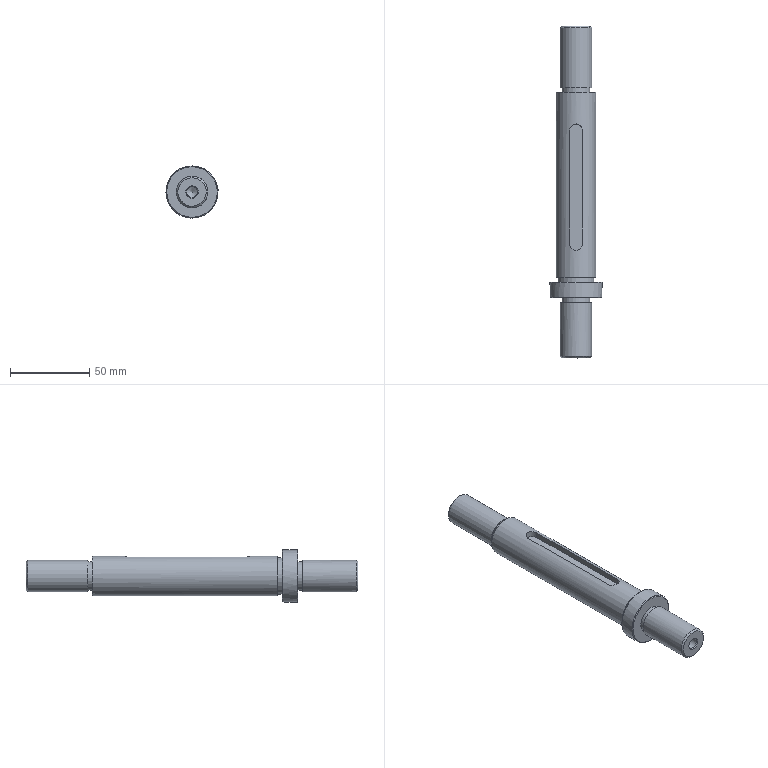Part | STEP file | YBQDJ-YB-16 | 1 solid | 30 faces | box 33 x 210 x 33 mm | volume 88192 mm3 | plane 11 | cylinder 11 | cone 8 | commonest cylinder face diameters 6.8 x2 8.04 x2 18 x2 20 x2 23 x1 25 x1